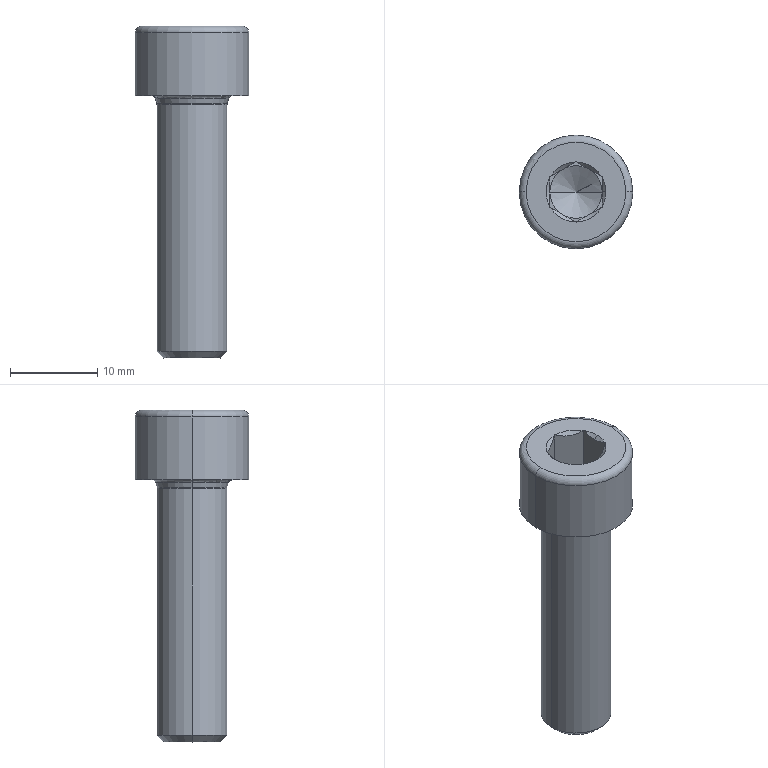Part | NX | features 2_12 2 | 1 solid | 38 faces | box 13 x 13 x 38 mm | volume 2398 mm3 | plane 15 | cone 13 | torus 6 | cylinder 4 | commonest cylinder face diameters 8 x2 13 x2
STEP:
#1=CARTESIAN_POINT('',(-141.767,-145.,-837.129));
#2=VERTEX_POINT('',#1);
#3=CARTESIAN_POINT('',(-148.233,-145.,-837.129));
#4=VERTEX_POINT('',#3);
#5=CARTESIAN_POINT('',(-145.,-145.,-837.129));
#6=DIRECTION('',(0.,0.,-1.));
#7=DIRECTION('',(1.,0.,0.));
#8=AXIS2_PLACEMENT_3D('',#5,#6,#7);
#9=CIRCLE('',#8,3.233);
#10=EDGE_CURVE('',#2,#4,#9,.T.);
#11=ORIENTED_EDGE('',*,*,#10,.F.);
#12=CARTESIAN_POINT('',(-141.,-145.,-836.362));
#13=VERTEX_POINT('',#12);
#14=CARTESIAN_POINT('',(-141.,-145.,-836.362));
#15=DIRECTION('',(-0.7071,0.,-0.7071));
#16=VECTOR('',#15,1000.);
#17=LINE('',#14,#16);
#18=EDGE_CURVE('',#13,#2,#17,.T.);
#19=ORIENTED_EDGE('',*,*,#18,.F.);
#20=CARTESIAN_POINT('',(-149.,-145.,-836.362));
#21=VERTEX_POINT('',#20);
#22=CARTESIAN_POINT('',(-145.,-145.,-836.362));
#23=DIRECTION('',(0.,0.,-1.));
#24=DIRECTION('',(1.,0.,0.));
#25=AXIS2_PLACEMENT_3D('',#22,#23,#24);
#26=CIRCLE('',#25,4.);
#27=EDGE_CURVE('',#13,#21,#26,.T.);
#28=ORIENTED_EDGE('',*,*,#27,.T.);
#29=CARTESIAN_POINT('',(-149.,-145.,-836.362));
#30=DIRECTION('',(0.7071,0.,-0.7071));
#31=VECTOR('',#30,1000.);
#32=LINE('',#29,#31);
#33=EDGE_CURVE('',#4,#21,#32,.F.);
#34=ORIENTED_EDGE('',*,*,#33,.F.);
#35=EDGE_LOOP('',(#11,#19,#28,#34));
#36=FACE_BOUND('',#35,.T.);
#37=CARTESIAN_POINT('',(-145.,-145.,-837.165));
#38=DIRECTION('',(0.,0.,1.));
#39=DIRECTION('',(1.,0.,0.));
#40=AXIS2_PLACEMENT_3D('',#37,#38,#39);
#41=CONICAL_SURFACE('',#40,3.197,0.7854);
#42=ADVANCED_FACE('',(#36),#41,.T.);
#43=ORIENTED_EDGE('',*,*,#10,.T.);
#44=CARTESIAN_POINT('',(-145.,-145.,-837.129));
#45=DIRECTION('',(0.,0.,-1.));
#46=DIRECTION('',(-1.,0.,0.));
#47=AXIS2_PLACEMENT_3D('',#44,#45,#46);
#48=CIRCLE('',#47,3.233);
#49=EDGE_CURVE('',#4,#2,#48,.T.);
#50=ORIENTED_EDGE('',*,*,#49,.T.);
#51=EDGE_LOOP('',(#43,#50));
#52=FACE_BOUND('',#51,.T.);
#53=CARTESIAN_POINT('',(-145.,-146.617,-837.129));
#54=DIRECTION('',(0.,0.,-1.));
#55=DIRECTION('',(-1.,0.,0.));
#56=AXIS2_PLACEMENT_3D('',#53,#54,#55);
#57=PLANE('',#56);
#58=ADVANCED_FACE('',(#52),#57,.T.);
#59=ORIENTED_EDGE('',*,*,#33,.T.);
#60=CARTESIAN_POINT('',(-145.,-145.,-836.362));
#61=DIRECTION('',(0.,0.,-1.));
#62=DIRECTION('',(-1.,0.,0.));
#63=AXIS2_PLACEMENT_3D('',#60,#61,#62);
#64=CIRCLE('',#63,4.);
#65=EDGE_CURVE('',#21,#13,#64,.T.);
#66=ORIENTED_EDGE('',*,*,#65,.T.);
#67=ORIENTED_EDGE('',*,*,#18,.T.);
#68=ORIENTED_EDGE('',*,*,#49,.F.);
#69=EDGE_LOOP('',(#59,#66,#67,#68));
#70=FACE_BOUND('',#69,.T.);
#71=CARTESIAN_POINT('',(-145.,-145.,-837.165));
#72=DIRECTION('',(0.,0.,1.));
#73=DIRECTION('',(1.,0.,0.));
#74=AXIS2_PLACEMENT_3D('',#71,#72,#73);
#75=CONICAL_SURFACE('',#74,3.197,0.7854);
#76=ADVANCED_FACE('',(#70),#75,.T.);
#77=CARTESIAN_POINT('',(-144.94,-141.571,-799.129));
#78=VERTEX_POINT('',#77);
#79=CARTESIAN_POINT('',(-142.06,-143.233,-799.129));
#80=VERTEX_POINT('',#79);
#81=CARTESIAN_POINT('',(-144.94,-141.571,-799.129));
#82=CARTESIAN_POINT('',(-144.491,-141.83,-799.381));
#83=CARTESIAN_POINT('',(-143.5,-142.402,-799.738));
#84=CARTESIAN_POINT('',(-142.509,-142.974,-799.381));
#85=CARTESIAN_POINT('',(-142.06,-143.233,-799.129));
#86=B_SPLINE_CURVE_WITH_KNOTS('',3,(#81,#82,#83,#84,#85),.UNSPECIFIED.,.F.,.F.,(4,1,4),(0.,0.5,1.),.UNSPECIFIED.);
#87=EDGE_CURVE('',#78,#80,#86,.T.);
#88=ORIENTED_EDGE('',*,*,#87,.T.);
#89=CARTESIAN_POINT('',(-145.,-145.,-799.129));
#90=DIRECTION('',(0.,0.,-1.));
#91=DIRECTION('',(0.01749,0.9998,0.));
#92=AXIS2_PLACEMENT_3D('',#89,#90,#91);
#93=CIRCLE('',#92,3.43);
#94=EDGE_CURVE('',#78,#80,#93,.T.);
#95=ORIENTED_EDGE('',*,*,#94,.F.);
#96=EDGE_LOOP('',(#88,#95));
#97=FACE_BOUND('',#96,.T.);
#98=CARTESIAN_POINT('',(-145.,-145.,-799.598));
#99=DIRECTION('',(0.,0.,1.));
#100=DIRECTION('',(1.,0.,0.));
#101=AXIS2_PLACEMENT_3D('',#98,#99,#100);
#102=CONICAL_SURFACE('',#101,2.962,0.7854);
#103=ADVANCED_FACE('',(#97),#102,.F.);
#104=CARTESIAN_POINT('',(-147.94,-143.233,-799.129));
#105=VERTEX_POINT('',#104);
#106=CARTESIAN_POINT('',(-145.06,-141.571,-799.129));
#107=VERTEX_POINT('',#106);
#108=CARTESIAN_POINT('',(-147.94,-143.233,-799.129));
#109=CARTESIAN_POINT('',(-147.491,-142.974,-799.381));
#110=CARTESIAN_POINT('',(-146.5,-142.402,-799.738));
#111=CARTESIAN_POINT('',(-145.509,-141.83,-799.381));
#112=CARTESIAN_POINT('',(-145.06,-141.571,-799.129));
#113=B_SPLINE_CURVE_WITH_KNOTS('',3,(#108,#109,#110,#111,#112),.UNSPECIFIED.,.F.,.F.,(4,1,4),(0.,0.5,1.),.UNSPECIFIED.);
#114=EDGE_CURVE('',#105,#107,#113,.T.);
#115=ORIENTED_EDGE('',*,*,#114,.T.);
#116=CARTESIAN_POINT('',(-145.,-145.,-799.129));
#117=DIRECTION('',(0.,0.,-1.));
#118=DIRECTION('',(-0.8572,0.5151,0.));
#119=AXIS2_PLACEMENT_3D('',#116,#117,#118);
#120=CIRCLE('',#119,3.43);
#121=EDGE_CURVE('',#105,#107,#120,.T.);
#122=ORIENTED_EDGE('',*,*,#121,.F.);
#123=EDGE_LOOP('',(#115,#122));
#124=FACE_BOUND('',#123,.T.);
#125=CARTESIAN_POINT('',(-145.,-145.,-799.598));
#126=DIRECTION('',(0.,0.,1.));
#127=DIRECTION('',(1.,0.,0.));
#128=AXIS2_PLACEMENT_3D('',#125,#126,#127);
#129=CONICAL_SURFACE('',#128,2.962,0.7854);
#130=ADVANCED_FACE('',(#124),#129,.F.);
#131=CARTESIAN_POINT('',(-145.,-141.536,-803.829));
#132=VERTEX_POINT('',#131);
#133=CARTESIAN_POINT('',(-146.5,-142.402,-803.829));
#134=VERTEX_POINT('',#133);
#135=CARTESIAN_POINT('',(-145.,-141.536,-803.829));
#136=DIRECTION('',(-0.866,-0.5,0.));
#137=VECTOR('',#136,1000.);
#138=LINE('',#135,#137);
#139=EDGE_CURVE('',#132,#134,#138,.T.);
#140=ORIENTED_EDGE('',*,*,#139,.T.);
#141=CARTESIAN_POINT('',(-143.5,-142.402,-803.829));
#142=VERTEX_POINT('',#141);
#143=CARTESIAN_POINT('',(-145.,-145.,-803.829));
#144=DIRECTION('',(0.,0.,-1.));
#145=DIRECTION('',(-0.5,0.866,0.));
#146=AXIS2_PLACEMENT_3D('',#143,#144,#145);
#147=CIRCLE('',#146,3.);
#148=EDGE_CURVE('',#134,#142,#147,.T.);
#149=ORIENTED_EDGE('',*,*,#148,.T.);
#150=CARTESIAN_POINT('',(-143.5,-142.402,-803.829));
#151=DIRECTION('',(-0.866,0.5,0.));
#152=VECTOR('',#151,1000.);
#153=LINE('',#150,#152);
#154=EDGE_CURVE('',#142,#132,#153,.T.);
#155=ORIENTED_EDGE('',*,*,#154,.T.);
#156=EDGE_LOOP('',(#140,#149,#155));
#157=FACE_BOUND('',#156,.T.);
#158=CARTESIAN_POINT('',(-145.,-145.,-803.829));
#159=DIRECTION('',(0.,0.,-1.));
#160=DIRECTION('',(-1.,0.,0.));
#161=AXIS2_PLACEMENT_3D('',#158,#159,#160);
#162=PLANE('',#161);
#163=ADVANCED_FACE('',(#157),#162,.F.);
#164=CARTESIAN_POINT('',(-145.,-148.464,-803.829));
#165=VERTEX_POINT('',#164);
#166=CARTESIAN_POINT('',(-143.5,-147.598,-803.829));
#167=VERTEX_POINT('',#166);
#168=CARTESIAN_POINT('',(-145.,-148.464,-803.829));
#169=DIRECTION('',(0.866,0.5,0.));
#170=VECTOR('',#169,1000.);
#171=LINE('',#168,#170);
#172=EDGE_CURVE('',#165,#167,#171,.T.);
#173=ORIENTED_EDGE('',*,*,#172,.T.);
#174=CARTESIAN_POINT('',(-146.5,-147.598,-803.829));
#175=VERTEX_POINT('',#174);
#176=CARTESIAN_POINT('',(-145.,-145.,-803.829));
#177=DIRECTION('',(0.,0.,-1.));
#178=DIRECTION('',(0.5,-0.866,0.));
#179=AXIS2_PLACEMENT_3D('',#176,#177,#178);
#180=CIRCLE('',#179,3.);
#181=EDGE_CURVE('',#167,#175,#180,.T.);
#182=ORIENTED_EDGE('',*,*,#181,.T.);
#183=CARTESIAN_POINT('',(-146.5,-147.598,-803.829));
#184=DIRECTION('',(0.866,-0.5,0.));
#185=VECTOR('',#184,1000.);
#186=LINE('',#183,#185);
#187=EDGE_CURVE('',#175,#165,#186,.T.);
#188=ORIENTED_EDGE('',*,*,#187,.T.);
#189=EDGE_LOOP('',(#173,#182,#188));
#190=FACE_BOUND('',#189,.T.);
#191=CARTESIAN_POINT('',(-145.,-145.,-803.829));
#192=DIRECTION('',(0.,0.,-1.));
#193=DIRECTION('',(-1.,0.,0.));
#194=AXIS2_PLACEMENT_3D('',#191,#192,#193);
#195=PLANE('',#194);
#196=ADVANCED_FACE('',(#190),#195,.F.);
#197=CARTESIAN_POINT('',(-148.,-146.732,-803.829));
#198=VERTEX_POINT('',#197);
#199=CARTESIAN_POINT('',(-148.,-146.732,-803.829));
#200=DIRECTION('',(0.866,-0.5,0.));
#201=VECTOR('',#200,1000.);
#202=LINE('',#199,#201);
#203=EDGE_CURVE('',#198,#175,#202,.T.);
#204=ORIENTED_EDGE('',*,*,#203,.T.);
#205=CARTESIAN_POINT('',(-148.,-145.,-803.829));
#206=VERTEX_POINT('',#205);
#207=CARTESIAN_POINT('',(-145.,-145.,-803.829));
#208=DIRECTION('',(0.,0.,-1.));
#209=DIRECTION('',(-0.5,-0.866,0.));
#210=AXIS2_PLACEMENT_3D('',#207,#208,#209);
#211=CIRCLE('',#210,3.);
#212=EDGE_CURVE('',#175,#206,#211,.T.);
#213=ORIENTED_EDGE('',*,*,#212,.T.);
#214=CARTESIAN_POINT('',(-148.,-145.,-803.829));
#215=DIRECTION('',(0.,-1.,0.));
#216=VECTOR('',#215,1000.);
#217=LINE('',#214,#216);
#218=EDGE_CURVE('',#206,#198,#217,.T.);
#219=ORIENTED_EDGE('',*,*,#218,.T.);
#220=EDGE_LOOP('',(#204,#213,#219));
#221=FACE_BOUND('',#220,.T.);
#222=CARTESIAN_POINT('',(-145.,-145.,-803.829));
#223=DIRECTION('',(0.,0.,-1.));
#224=DIRECTION('',(-1.,0.,0.));
#225=AXIS2_PLACEMENT_3D('',#222,#223,#224);
#226=PLANE('',#225);
#227=ADVANCED_FACE('',(#221),#226,.F.);
#228=CARTESIAN_POINT('',(-145.06,-148.429,-799.129));
#229=VERTEX_POINT('',#228);
#230=CARTESIAN_POINT('',(-147.94,-146.767,-799.129));
#231=VERTEX_POINT('',#230);
#232=CARTESIAN_POINT('',(-145.,-145.,-799.129));
#233=DIRECTION('',(0.,0.,-1.));
#234=DIRECTION('',(-0.01749,-0.9998,0.));
#235=AXIS2_PLACEMENT_3D('',#232,#233,#234);
#236=CIRCLE('',#235,3.43);
#237=EDGE_CURVE('',#229,#231,#236,.T.);
#238=ORIENTED_EDGE('',*,*,#237,.F.);
#239=CARTESIAN_POINT('',(-145.06,-148.429,-799.129));
#240=CARTESIAN_POINT('',(-145.509,-148.17,-799.381));
#241=CARTESIAN_POINT('',(-146.5,-147.598,-799.738));
#242=CARTESIAN_POINT('',(-147.491,-147.026,-799.381));
#243=CARTESIAN_POINT('',(-147.94,-146.767,-799.129));
#244=B_SPLINE_CURVE_WITH_KNOTS('',3,(#239,#240,#241,#242,#243),.UNSPECIFIED.,.F.,.F.,(4,1,4),(0.,0.5,1.),.UNSPECIFIED.);
#245=EDGE_CURVE('',#229,#231,#244,.T.);
#246=ORIENTED_EDGE('',*,*,#245,.T.);
#247=EDGE_LOOP('',(#238,#246));
#248=FACE_BOUND('',#247,.T.);
#249=CARTESIAN_POINT('',(-145.,-145.,-799.598));
#250=DIRECTION('',(0.,0.,1.));
#251=DIRECTION('',(1.,0.,0.));
#252=AXIS2_PLACEMENT_3D('',#249,#250,#251);
#253=CONICAL_SURFACE('',#252,2.962,0.7854);
#254=ADVANCED_FACE('',(#248),#253,.F.);
#255=ORIENTED_EDGE('',*,*,#187,.F.);
#256=ORIENTED_EDGE('',*,*,#203,.F.);
#257=CARTESIAN_POINT('',(-148.,-146.732,-799.129));
#258=VERTEX_POINT('',#257);
#259=CARTESIAN_POINT('',(-148.,-146.732,-799.129));
#260=DIRECTION('',(0.,0.,-1.));
#261=VECTOR('',#260,1000.);
#262=LINE('',#259,#261);
#263=EDGE_CURVE('',#258,#198,#262,.T.);
#264=ORIENTED_EDGE('',*,*,#263,.F.);
#265=CARTESIAN_POINT('',(-147.94,-146.767,-799.129));
#266=DIRECTION('',(-0.866,0.5,0.));
#267=VECTOR('',#266,1000.);
#268=LINE('',#265,#267);
#269=EDGE_CURVE('',#231,#258,#268,.T.);
#270=ORIENTED_EDGE('',*,*,#269,.F.);
#271=ORIENTED_EDGE('',*,*,#245,.F.);
#272=CARTESIAN_POINT('',(-145.,-148.464,-799.129));
#273=VERTEX_POINT('',#272);
#274=CARTESIAN_POINT('',(-145.,-148.464,-799.129));
#275=DIRECTION('',(-0.866,0.5,0.));
#276=VECTOR('',#275,1000.);
#277=LINE('',#274,#276);
#278=EDGE_CURVE('',#273,#229,#277,.T.);
#279=ORIENTED_EDGE('',*,*,#278,.F.);
#280=CARTESIAN_POINT('',(-145.,-148.464,-799.129));
#281=DIRECTION('',(0.,0.,-1.));
#282=VECTOR('',#281,1000.);
#283=LINE('',#280,#282);
#284=EDGE_CURVE('',#273,#165,#283,.T.);
#285=ORIENTED_EDGE('',*,*,#284,.T.);
#286=EDGE_LOOP('',(#255,#256,#264,#270,#271,#279,#285));
#287=FACE_BOUND('',#286,.T.);
#288=CARTESIAN_POINT('',(-145.,-148.464,-803.829));
#289=DIRECTION('',(-0.5,-0.866,0.));
#290=DIRECTION('',(0.866,-0.5,0.));
#291=AXIS2_PLACEMENT_3D('',#288,#289,#290);
#292=PLANE('',#291);
#293=ADVANCED_FACE('',(#287),#292,.F.);
#294=CARTESIAN_POINT('',(-142.06,-146.767,-799.129));
#295=VERTEX_POINT('',#294);
#296=CARTESIAN_POINT('',(-144.94,-148.429,-799.129));
#297=VERTEX_POINT('',#296);
#298=CARTESIAN_POINT('',(-145.,-145.,-799.129));
#299=DIRECTION('',(0.,0.,-1.));
#300=DIRECTION('',(0.8572,-0.5151,0.));
#301=AXIS2_PLACEMENT_3D('',#298,#299,#300);
#302=CIRCLE('',#301,3.43);
#303=EDGE_CURVE('',#295,#297,#302,.T.);
#304=ORIENTED_EDGE('',*,*,#303,.F.);
#305=CARTESIAN_POINT('',(-142.06,-146.767,-799.129));
#306=CARTESIAN_POINT('',(-142.509,-147.026,-799.381));
#307=CARTESIAN_POINT('',(-143.5,-147.598,-799.738));
#308=CARTESIAN_POINT('',(-144.491,-148.17,-799.381));
#309=CARTESIAN_POINT('',(-144.94,-148.429,-799.129));
#310=B_SPLINE_CURVE_WITH_KNOTS('',3,(#305,#306,#307,#308,#309),.UNSPECIFIED.,.F.,.F.,(4,1,4),(0.,0.5,1.),.UNSPECIFIED.);
#311=EDGE_CURVE('',#295,#297,#310,.T.);
#312=ORIENTED_EDGE('',*,*,#311,.T.);
#313=EDGE_LOOP('',(#304,#312));
#314=FACE_BOUND('',#313,.T.);
#315=CARTESIAN_POINT('',(-145.,-145.,-799.598));
#316=DIRECTION('',(0.,0.,1.));
#317=DIRECTION('',(1.,0.,0.));
#318=AXIS2_PLACEMENT_3D('',#315,#316,#317);
#319=CONICAL_SURFACE('',#318,2.962,0.7854);
#320=ADVANCED_FACE('',(#314),#319,.F.);
#321=CARTESIAN_POINT('',(-142.,-143.268,-803.829));
#322=VERTEX_POINT('',#321);
#323=CARTESIAN_POINT('',(-142.,-143.268,-803.829));
#324=DIRECTION('',(-0.866,0.5,0.));
#325=VECTOR('',#324,1000.);
#326=LINE('',#323,#325);
#327=EDGE_CURVE('',#322,#142,#326,.T.);
#328=ORIENTED_EDGE('',*,*,#327,.T.);
#329=CARTESIAN_POINT('',(-142.,-145.,-803.829));
#330=VERTEX_POINT('',#329);
#331=CARTESIAN_POINT('',(-145.,-145.,-803.829));
#332=DIRECTION('',(0.,0.,-1.));
#333=DIRECTION('',(0.5,0.866,0.));
#334=AXIS2_PLACEMENT_3D('',#331,#332,#333);
#335=CIRCLE('',#334,3.);
#336=EDGE_CURVE('',#142,#330,#335,.T.);
#337=ORIENTED_EDGE('',*,*,#336,.T.);
#338=CARTESIAN_POINT('',(-142.,-145.,-803.829));
#339=DIRECTION('',(0.,1.,0.));
#340=VECTOR('',#339,1000.);
#341=LINE('',#338,#340);
#342=EDGE_CURVE('',#330,#322,#341,.T.);
#343=ORIENTED_EDGE('',*,*,#342,.T.);
#344=EDGE_LOOP('',(#328,#337,#343));
#345=FACE_BOUND('',#344,.T.);
#346=CARTESIAN_POINT('',(-145.,-145.,-803.829));
#347=DIRECTION('',(0.,0.,-1.));
#348=DIRECTION('',(-1.,0.,0.));
#349=AXIS2_PLACEMENT_3D('',#346,#347,#348);
#350=PLANE('',#349);
#351=ADVANCED_FACE('',(#345),#350,.F.);
#352=CARTESIAN_POINT('',(-142.,-145.,-799.559));
#353=VERTEX_POINT('',#352);
#354=CARTESIAN_POINT('',(-142.,-146.663,-799.129));
#355=VERTEX_POINT('',#354);
#356=CARTESIAN_POINT('',(-142.,-145.,-799.559));
#357=CARTESIAN_POINT('',(-142.,-145.578,-799.561));
#358=CARTESIAN_POINT('',(-142.,-146.144,-799.381));
#359=CARTESIAN_POINT('',(-142.,-146.663,-799.129));
#360=B_SPLINE_CURVE_WITH_KNOTS('',3,(#356,#357,#358,#359),.UNSPECIFIED.,.F.,.F.,(4,4),(0.,1.),.UNSPECIFIED.);
#361=EDGE_CURVE('',#353,#355,#360,.T.);
#362=ORIENTED_EDGE('',*,*,#361,.T.);
#363=CARTESIAN_POINT('',(-141.57,-145.,-799.129));
#364=VERTEX_POINT('',#363);
#365=CARTESIAN_POINT('',(-145.,-145.,-799.129));
#366=DIRECTION('',(0.,0.,-1.));
#367=DIRECTION('',(1.,0.,0.));
#368=AXIS2_PLACEMENT_3D('',#365,#366,#367);
#369=CIRCLE('',#368,3.43);
#370=EDGE_CURVE('',#364,#355,#369,.T.);
#371=ORIENTED_EDGE('',*,*,#370,.F.);
#372=CARTESIAN_POINT('',(-141.57,-145.,-799.129));
#373=DIRECTION('',(-0.7071,0.,-0.7071));
#374=VECTOR('',#373,1000.);
#375=LINE('',#372,#374);
#376=EDGE_CURVE('',#364,#353,#375,.T.);
#377=ORIENTED_EDGE('',*,*,#376,.T.);
#378=EDGE_LOOP('',(#362,#371,#377));
#379=FACE_BOUND('',#378,.T.);
#380=CARTESIAN_POINT('',(-145.,-145.,-799.595));
#381=DIRECTION('',(0.,0.,1.));
#382=DIRECTION('',(1.,0.,0.));
#383=AXIS2_PLACEMENT_3D('',#380,#381,#382);
#384=CONICAL_SURFACE('',#383,2.964,0.7854);
#385=ADVANCED_FACE('',(#379),#384,.F.);
#386=ORIENTED_EDGE('',*,*,#376,.F.);
#387=CARTESIAN_POINT('',(-142.,-143.337,-799.129));
#388=VERTEX_POINT('',#387);
#389=CARTESIAN_POINT('',(-145.,-145.,-799.129));
#390=DIRECTION('',(0.,0.,-1.));
#391=DIRECTION('',(0.8746,0.4848,0.));
#392=AXIS2_PLACEMENT_3D('',#389,#390,#391);
#393=CIRCLE('',#392,3.43);
#394=EDGE_CURVE('',#388,#364,#393,.T.);
#395=ORIENTED_EDGE('',*,*,#394,.F.);
#396=CARTESIAN_POINT('',(-142.,-143.337,-799.129));
#397=CARTESIAN_POINT('',(-142.,-143.856,-799.381));
#398=CARTESIAN_POINT('',(-142.,-144.422,-799.56));
#399=CARTESIAN_POINT('',(-142.,-145.,-799.559));
#400=B_SPLINE_CURVE_WITH_KNOTS('',3,(#396,#397,#398,#399),.UNSPECIFIED.,.F.,.F.,(4,4),(0.,1.),.UNSPECIFIED.);
#401=EDGE_CURVE('',#388,#353,#400,.T.);
#402=ORIENTED_EDGE('',*,*,#401,.T.);
#403=EDGE_LOOP('',(#386,#395,#402));
#404=FACE_BOUND('',#403,.T.);
#405=CARTESIAN_POINT('',(-145.,-145.,-799.595));
#406=DIRECTION('',(0.,0.,1.));
#407=DIRECTION('',(1.,0.,0.));
#408=AXIS2_PLACEMENT_3D('',#405,#406,#407);
#409=CONICAL_SURFACE('',#408,2.964,0.7854);
#410=ADVANCED_FACE('',(#404),#409,.F.);
#411=ORIENTED_EDGE('',*,*,#342,.F.);
#412=CARTESIAN_POINT('',(-142.,-146.732,-803.829));
#413=VERTEX_POINT('',#412);
#414=CARTESIAN_POINT('',(-142.,-145.,-803.829));
#415=DIRECTION('',(0.,-1.,0.));
#416=VECTOR('',#415,1000.);
#417=LINE('',#414,#416);
#418=EDGE_CURVE('',#330,#413,#417,.T.);
#419=ORIENTED_EDGE('',*,*,#418,.T.);
#420=CARTESIAN_POINT('',(-142.,-146.732,-799.129));
#421=VERTEX_POINT('',#420);
#422=CARTESIAN_POINT('',(-142.,-146.732,-799.129));
#423=DIRECTION('',(0.,0.,-1.));
#424=VECTOR('',#423,1000.);
#425=LINE('',#422,#424);
#426=EDGE_CURVE('',#421,#413,#425,.T.);
#427=ORIENTED_EDGE('',*,*,#426,.F.);
#428=CARTESIAN_POINT('',(-142.,-146.732,-799.129));
#429=DIRECTION('',(0.,1.,0.));
#430=VECTOR('',#429,1000.);
#431=LINE('',#428,#430);
#432=EDGE_CURVE('',#421,#355,#431,.T.);
#433=ORIENTED_EDGE('',*,*,#432,.T.);
#434=ORIENTED_EDGE('',*,*,#361,.F.);
#435=ORIENTED_EDGE('',*,*,#401,.F.);
#436=CARTESIAN_POINT('',(-142.,-143.268,-799.129));
#437=VERTEX_POINT('',#436);
#438=CARTESIAN_POINT('',(-142.,-143.337,-799.129));
#439=DIRECTION('',(0.,1.,0.));
#440=VECTOR('',#439,1000.);
#441=LINE('',#438,#440);
#442=EDGE_CURVE('',#388,#437,#441,.T.);
#443=ORIENTED_EDGE('',*,*,#442,.T.);
#444=CARTESIAN_POINT('',(-142.,-143.268,-803.829));
#445=DIRECTION('',(0.,0.,1.));
#446=VECTOR('',#445,1000.);
#447=LINE('',#444,#446);
#448=EDGE_CURVE('',#322,#437,#447,.T.);
#449=ORIENTED_EDGE('',*,*,#448,.F.);
#450=EDGE_LOOP('',(#411,#419,#427,#433,#434,#435,#443,#449));
#451=FACE_BOUND('',#450,.T.);
#452=CARTESIAN_POINT('',(-142.,-143.268,-803.829));
#453=DIRECTION('',(1.,0.,0.));
#454=DIRECTION('',(0.,0.,-1.));
#455=AXIS2_PLACEMENT_3D('',#452,#453,#454);
#456=PLANE('',#455);
#457=ADVANCED_FACE('',(#451),#456,.F.);
#458=CARTESIAN_POINT('',(-143.5,-147.598,-803.829));
#459=DIRECTION('',(0.866,0.5,0.));
#460=VECTOR('',#459,1000.);
#461=LINE('',#458,#460);
#462=EDGE_CURVE('',#167,#413,#461,.T.);
#463=ORIENTED_EDGE('',*,*,#462,.F.);
#464=ORIENTED_EDGE('',*,*,#172,.F.);
#465=ORIENTED_EDGE('',*,*,#284,.F.);
#466=CARTESIAN_POINT('',(-144.94,-148.429,-799.129));
#467=DIRECTION('',(-0.866,-0.5,0.));
#468=VECTOR('',#467,1000.);
#469=LINE('',#466,#468);
#470=EDGE_CURVE('',#297,#273,#469,.T.);
#471=ORIENTED_EDGE('',*,*,#470,.F.);
#472=ORIENTED_EDGE('',*,*,#311,.F.);
#473=CARTESIAN_POINT('',(-142.,-146.732,-799.129));
#474=DIRECTION('',(-0.866,-0.5,0.));
#475=VECTOR('',#474,1000.);
#476=LINE('',#473,#475);
#477=EDGE_CURVE('',#421,#295,#476,.T.);
#478=ORIENTED_EDGE('',*,*,#477,.F.);
#479=ORIENTED_EDGE('',*,*,#426,.T.);
#480=EDGE_LOOP('',(#463,#464,#465,#471,#472,#478,#479));
#481=FACE_BOUND('',#480,.T.);
#482=CARTESIAN_POINT('',(-142.,-146.732,-803.829));
#483=DIRECTION('',(0.5,-0.866,0.));
#484=DIRECTION('',(0.866,0.5,0.));
#485=AXIS2_PLACEMENT_3D('',#482,#483,#484);
#486=PLANE('',#485);
#487=ADVANCED_FACE('',(#481),#486,.F.);
#488=ORIENTED_EDGE('',*,*,#418,.F.);
#489=CARTESIAN_POINT('',(-145.,-145.,-803.829));
#490=DIRECTION('',(0.,0.,-1.));
#491=DIRECTION('',(1.,0.,0.));
#492=AXIS2_PLACEMENT_3D('',#489,#490,#491);
#493=CIRCLE('',#492,3.);
#494=EDGE_CURVE('',#330,#167,#493,.T.);
#495=ORIENTED_EDGE('',*,*,#494,.T.);
#496=ORIENTED_EDGE('',*,*,#462,.T.);
#497=EDGE_LOOP('',(#488,#495,#496));
#498=FACE_BOUND('',#497,.T.);
#499=CARTESIAN_POINT('',(-145.,-145.,-803.829));
#500=DIRECTION('',(0.,0.,-1.));
#501=DIRECTION('',(-1.,0.,0.));
#502=AXIS2_PLACEMENT_3D('',#499,#500,#501);
#503=PLANE('',#502);
#504=ADVANCED_FACE('',(#498),#503,.F.);
#505=CARTESIAN_POINT('',(-145.,-145.,-805.561));
#506=VERTEX_POINT('',#505);
#507=CARTESIAN_POINT('',(-148.,-145.,-803.829));
#508=DIRECTION('',(0.866,0.,-0.5));
#509=VECTOR('',#508,1000.);
#510=LINE('',#507,#509);
#511=EDGE_CURVE('',#206,#506,#510,.T.);
#512=ORIENTED_EDGE('',*,*,#511,.F.);
#513=ORIENTED_EDGE('',*,*,#212,.F.);
#514=ORIENTED_EDGE('',*,*,#181,.F.);
#515=ORIENTED_EDGE('',*,*,#494,.F.);
#516=CARTESIAN_POINT('',(-142.,-145.,-803.829));
#517=DIRECTION('',(-0.866,0.,-0.5));
#518=VECTOR('',#517,1000.);
#519=LINE('',#516,#518);
#520=EDGE_CURVE('',#506,#330,#519,.F.);
#521=ORIENTED_EDGE('',*,*,#520,.F.);
#522=EDGE_LOOP('',(#512,#513,#514,#515,#521));
#523=FACE_BOUND('',#522,.T.);
#524=CARTESIAN_POINT('',(-145.,-145.,-805.561));
#525=DIRECTION('',(0.,0.,1.));
#526=DIRECTION('',(1.,0.,0.));
#527=AXIS2_PLACEMENT_3D('',#524,#525,#526);
#528=CONICAL_SURFACE('',#527,0.,1.047);
#529=ADVANCED_FACE('',(#523),#528,.F.);
#530=ORIENTED_EDGE('',*,*,#520,.T.);
#531=ORIENTED_EDGE('',*,*,#336,.F.);
#532=ORIENTED_EDGE('',*,*,#148,.F.);
#533=CARTESIAN_POINT('',(-145.,-145.,-803.829));
#534=DIRECTION('',(0.,0.,-1.));
#535=DIRECTION('',(-1.,0.,0.));
#536=AXIS2_PLACEMENT_3D('',#533,#534,#535);
#537=CIRCLE('',#536,3.);
#538=EDGE_CURVE('',#206,#134,#537,.T.);
#539=ORIENTED_EDGE('',*,*,#538,.F.);
#540=ORIENTED_EDGE('',*,*,#511,.T.);
#541=EDGE_LOOP('',(#530,#531,#532,#539,#540));
#542=FACE_BOUND('',#541,.T.);
#543=CARTESIAN_POINT('',(-145.,-145.,-805.561));
#544=DIRECTION('',(0.,0.,1.));
#545=DIRECTION('',(1.,0.,0.));
#546=AXIS2_PLACEMENT_3D('',#543,#544,#545);
#547=CONICAL_SURFACE('',#546,0.,1.047);
#548=ADVANCED_FACE('',(#542),#547,.F.);
#549=CARTESIAN_POINT('',(-148.,-143.268,-803.829));
#550=VERTEX_POINT('',#549);
#551=CARTESIAN_POINT('',(-148.,-143.268,-803.829));
#552=DIRECTION('',(0.,-1.,0.));
#553=VECTOR('',#552,1000.);
#554=LINE('',#551,#553);
#555=EDGE_CURVE('',#550,#206,#554,.T.);
#556=ORIENTED_EDGE('',*,*,#555,.T.);
#557=ORIENTED_EDGE('',*,*,#538,.T.);
#558=CARTESIAN_POINT('',(-146.5,-142.402,-803.829));
#559=DIRECTION('',(-0.866,-0.5,0.));
#560=VECTOR('',#559,1000.);
#561=LINE('',#558,#560);
#562=EDGE_CURVE('',#134,#550,#561,.T.);
#563=ORIENTED_EDGE('',*,*,#562,.T.);
#564=EDGE_LOOP('',(#556,#557,#563));
#565=FACE_BOUND('',#564,.T.);
#566=CARTESIAN_POINT('',(-145.,-145.,-803.829));
#567=DIRECTION('',(0.,0.,-1.));
#568=DIRECTION('',(-1.,0.,0.));
#569=AXIS2_PLACEMENT_3D('',#566,#567,#568);
#570=PLANE('',#569);
#571=ADVANCED_FACE('',(#565),#570,.F.);
#572=CARTESIAN_POINT('',(-148.,-146.663,-799.129));
#573=VERTEX_POINT('',#572);
#574=CARTESIAN_POINT('',(-148.43,-145.,-799.129));
#575=VERTEX_POINT('',#574);
#576=CARTESIAN_POINT('',(-145.,-145.,-799.129));
#577=DIRECTION('',(0.,0.,-1.));
#578=DIRECTION('',(-0.8746,-0.4848,0.));
#579=AXIS2_PLACEMENT_3D('',#576,#577,#578);
#580=CIRCLE('',#579,3.43);
#581=EDGE_CURVE('',#573,#575,#580,.T.);
#582=ORIENTED_EDGE('',*,*,#581,.F.);
#583=CARTESIAN_POINT('',(-148.,-145.,-799.559));
#584=VERTEX_POINT('',#583);
#585=CARTESIAN_POINT('',(-148.,-146.663,-799.129));
#586=CARTESIAN_POINT('',(-148.,-146.144,-799.381));
#587=CARTESIAN_POINT('',(-148.,-145.578,-799.56));
#588=CARTESIAN_POINT('',(-148.,-145.,-799.559));
#589=B_SPLINE_CURVE_WITH_KNOTS('',3,(#585,#586,#587,#588),.UNSPECIFIED.,.F.,.F.,(4,4),(0.,1.),.UNSPECIFIED.);
#590=EDGE_CURVE('',#573,#584,#589,.T.);
#591=ORIENTED_EDGE('',*,*,#590,.T.);
#592=CARTESIAN_POINT('',(-148.,-143.337,-799.129));
#593=VERTEX_POINT('',#592);
#594=CARTESIAN_POINT('',(-148.,-145.,-799.559));
#595=CARTESIAN_POINT('',(-148.,-144.422,-799.561));
#596=CARTESIAN_POINT('',(-148.,-143.856,-799.381));
#597=CARTESIAN_POINT('',(-148.,-143.337,-799.129));
#598=B_SPLINE_CURVE_WITH_KNOTS('',3,(#594,#595,#596,#597),.UNSPECIFIED.,.F.,.F.,(4,4),(0.,1.),.UNSPECIFIED.);
#599=EDGE_CURVE('',#584,#593,#598,.T.);
#600=ORIENTED_EDGE('',*,*,#599,.T.);
#601=CARTESIAN_POINT('',(-145.,-145.,-799.129));
#602=DIRECTION('',(0.,0.,-1.));
#603=DIRECTION('',(-1.,0.,0.));
#604=AXIS2_PLACEMENT_3D('',#601,#602,#603);
#605=CIRCLE('',#604,3.43);
#606=EDGE_CURVE('',#575,#593,#605,.T.);
#607=ORIENTED_EDGE('',*,*,#606,.F.);
#608=EDGE_LOOP('',(#582,#591,#600,#607));
#609=FACE_BOUND('',#608,.T.);
#610=CARTESIAN_POINT('',(-145.,-145.,-799.595));
#611=DIRECTION('',(0.,0.,1.));
#612=DIRECTION('',(1.,0.,0.));
#613=AXIS2_PLACEMENT_3D('',#610,#611,#612);
#614=CONICAL_SURFACE('',#613,2.964,0.7854);
#615=ADVANCED_FACE('',(#609),#614,.F.);
#616=ORIENTED_EDGE('',*,*,#263,.T.);
#617=ORIENTED_EDGE('',*,*,#218,.F.);
#618=ORIENTED_EDGE('',*,*,#555,.F.);
#619=CARTESIAN_POINT('',(-148.,-143.268,-799.129));
#620=VERTEX_POINT('',#619);
#621=CARTESIAN_POINT('',(-148.,-143.268,-799.129));
#622=DIRECTION('',(0.,0.,-1.));
#623=VECTOR('',#622,1000.);
#624=LINE('',#621,#623);
#625=EDGE_CURVE('',#620,#550,#624,.T.);
#626=ORIENTED_EDGE('',*,*,#625,.F.);
#627=CARTESIAN_POINT('',(-148.,-143.268,-799.129));
#628=DIRECTION('',(0.,-1.,0.));
#629=VECTOR('',#628,1000.);
#630=LINE('',#627,#629);
#631=EDGE_CURVE('',#620,#593,#630,.T.);
#632=ORIENTED_EDGE('',*,*,#631,.T.);
#633=ORIENTED_EDGE('',*,*,#599,.F.);
#634=ORIENTED_EDGE('',*,*,#590,.F.);
#635=CARTESIAN_POINT('',(-148.,-146.663,-799.129));
#636=DIRECTION('',(0.,-1.,0.));
#637=VECTOR('',#636,1000.);
#638=LINE('',#635,#637);
#639=EDGE_CURVE('',#573,#258,#638,.T.);
#640=ORIENTED_EDGE('',*,*,#639,.T.);
#641=EDGE_LOOP('',(#616,#617,#618,#626,#632,#633,#634,#640));
#642=FACE_BOUND('',#641,.T.);
#643=CARTESIAN_POINT('',(-148.,-146.732,-803.829));
#644=DIRECTION('',(-1.,0.,0.));
#645=DIRECTION('',(0.,0.,1.));
#646=AXIS2_PLACEMENT_3D('',#643,#644,#645);
#647=PLANE('',#646);
#648=ADVANCED_FACE('',(#642),#647,.F.);
#649=ORIENTED_EDGE('',*,*,#562,.F.);
#650=ORIENTED_EDGE('',*,*,#139,.F.);
#651=CARTESIAN_POINT('',(-145.,-141.536,-799.129));
#652=VERTEX_POINT('',#651);
#653=CARTESIAN_POINT('',(-145.,-141.536,-799.129));
#654=DIRECTION('',(0.,0.,-1.));
#655=VECTOR('',#654,1000.);
#656=LINE('',#653,#655);
#657=EDGE_CURVE('',#652,#132,#656,.T.);
#658=ORIENTED_EDGE('',*,*,#657,.F.);
#659=CARTESIAN_POINT('',(-145.06,-141.571,-799.129));
#660=DIRECTION('',(0.866,0.5,0.));
#661=VECTOR('',#660,1000.);
#662=LINE('',#659,#661);
#663=EDGE_CURVE('',#107,#652,#662,.T.);
#664=ORIENTED_EDGE('',*,*,#663,.F.);
#665=ORIENTED_EDGE('',*,*,#114,.F.);
#666=CARTESIAN_POINT('',(-148.,-143.268,-799.129));
#667=DIRECTION('',(0.866,0.5,0.));
#668=VECTOR('',#667,1000.);
#669=LINE('',#666,#668);
#670=EDGE_CURVE('',#620,#105,#669,.T.);
#671=ORIENTED_EDGE('',*,*,#670,.F.);
#672=ORIENTED_EDGE('',*,*,#625,.T.);
#673=EDGE_LOOP('',(#649,#650,#658,#664,#665,#671,#672));
#674=FACE_BOUND('',#673,.T.);
#675=CARTESIAN_POINT('',(-148.,-143.268,-803.829));
#676=DIRECTION('',(-0.5,0.866,0.));
#677=DIRECTION('',(-0.866,-0.5,0.));
#678=AXIS2_PLACEMENT_3D('',#675,#676,#677);
#679=PLANE('',#678);
#680=ADVANCED_FACE('',(#674),#679,.F.);
#681=ORIENTED_EDGE('',*,*,#154,.F.);
#682=ORIENTED_EDGE('',*,*,#327,.F.);
#683=ORIENTED_EDGE('',*,*,#448,.T.);
#684=CARTESIAN_POINT('',(-142.06,-143.233,-799.129));
#685=DIRECTION('',(0.866,-0.5,0.));
#686=VECTOR('',#685,1000.);
#687=LINE('',#684,#686);
#688=EDGE_CURVE('',#80,#437,#687,.T.);
#689=ORIENTED_EDGE('',*,*,#688,.F.);
#690=ORIENTED_EDGE('',*,*,#87,.F.);
#691=CARTESIAN_POINT('',(-145.,-141.536,-799.129));
#692=DIRECTION('',(0.866,-0.5,0.));
#693=VECTOR('',#692,1000.);
#694=LINE('',#691,#693);
#695=EDGE_CURVE('',#652,#78,#694,.T.);
#696=ORIENTED_EDGE('',*,*,#695,.F.);
#697=ORIENTED_EDGE('',*,*,#657,.T.);
#698=EDGE_LOOP('',(#681,#682,#683,#689,#690,#696,#697));
#699=FACE_BOUND('',#698,.T.);
#700=CARTESIAN_POINT('',(-145.,-141.536,-803.829));
#701=DIRECTION('',(0.5,0.866,0.));
#702=DIRECTION('',(-0.866,0.5,0.));
#703=AXIS2_PLACEMENT_3D('',#700,#701,#702);
#704=PLANE('',#703);
#705=ADVANCED_FACE('',(#699),#704,.F.);
#706=CARTESIAN_POINT('',(-151.5,-145.,-799.929));
#707=VERTEX_POINT('',#706);
#708=CARTESIAN_POINT('',(-138.5,-145.,-799.929));
#709=VERTEX_POINT('',#708);
#710=CARTESIAN_POINT('',(-145.,-145.,-799.929));
#711=DIRECTION('',(0.,0.,1.));
#712=DIRECTION('',(-1.,0.,0.));
#713=AXIS2_PLACEMENT_3D('',#710,#711,#712);
#714=CIRCLE('',#713,6.5);
#715=EDGE_CURVE('',#707,#709,#714,.T.);
#716=ORIENTED_EDGE('',*,*,#715,.F.);
#717=CARTESIAN_POINT('',(-151.5,-145.,-807.129));
#718=VERTEX_POINT('',#717);
#719=CARTESIAN_POINT('',(-151.5,-145.,-807.129));
#720=DIRECTION('',(0.,0.,1.));
#721=VECTOR('',#720,1000.);
#722=LINE('',#719,#721);
#723=EDGE_CURVE('',#718,#707,#722,.T.);
#724=ORIENTED_EDGE('',*,*,#723,.F.);
#725=CARTESIAN_POINT('',(-138.5,-145.,-807.129));
#726=VERTEX_POINT('',#725);
#727=CARTESIAN_POINT('',(-145.,-145.,-807.129));
#728=DIRECTION('',(0.,0.,-1.));
#729=DIRECTION('',(1.,0.,0.));
#730=AXIS2_PLACEMENT_3D('',#727,#728,#729);
#731=CIRCLE('',#730,6.5);
#732=EDGE_CURVE('',#726,#718,#731,.T.);
#733=ORIENTED_EDGE('',*,*,#732,.F.);
#734=CARTESIAN_POINT('',(-138.5,-145.,-807.129));
#735=DIRECTION('',(0.,0.,1.));
#736=VECTOR('',#735,1000.);
#737=LINE('',#734,#736);
#738=EDGE_CURVE('',#709,#726,#737,.F.);
#739=ORIENTED_EDGE('',*,*,#738,.F.);
#740=EDGE_LOOP('',(#716,#724,#733,#739));
#741=FACE_BOUND('',#740,.T.);
#742=CARTESIAN_POINT('',(-145.,-145.,-803.529));
#743=DIRECTION('',(0.,0.,-1.));
#744=DIRECTION('',(-1.,0.,0.));
#745=AXIS2_PLACEMENT_3D('',#742,#743,#744);
#746=CYLINDRICAL_SURFACE('',#745,6.5);
#747=ADVANCED_FACE('',(#741),#746,.T.);
#748=CARTESIAN_POINT('',(-145.,-150.7,-799.129));
#749=VERTEX_POINT('',#748);
#750=CARTESIAN_POINT('',(-139.3,-145.,-799.129));
#751=VERTEX_POINT('',#750);
#752=CARTESIAN_POINT('',(-145.,-145.,-799.129));
#753=DIRECTION('',(0.,0.,1.));
#754=DIRECTION('',(0.,-1.,0.));
#755=AXIS2_PLACEMENT_3D('',#752,#753,#754);
#756=CIRCLE('',#755,5.7);
#757=EDGE_CURVE('',#749,#751,#756,.T.);
#758=ORIENTED_EDGE('',*,*,#757,.F.);
#759=CARTESIAN_POINT('',(-150.7,-145.,-799.129));
#760=VERTEX_POINT('',#759);
#761=CARTESIAN_POINT('',(-145.,-145.,-799.129));
#762=DIRECTION('',(0.,0.,1.));
#763=DIRECTION('',(-1.,0.,0.));
#764=AXIS2_PLACEMENT_3D('',#761,#762,#763);
#765=CIRCLE('',#764,5.7);
#766=EDGE_CURVE('',#760,#749,#765,.T.);
#767=ORIENTED_EDGE('',*,*,#766,.F.);
#768=CARTESIAN_POINT('',(-150.7,-145.,-799.929));
#769=DIRECTION('',(0.,1.,0.));
#770=DIRECTION('',(-1.,0.,0.));
#771=AXIS2_PLACEMENT_3D('',#768,#769,#770);
#772=CIRCLE('',#771,0.8);
#773=EDGE_CURVE('',#707,#760,#772,.T.);
#774=ORIENTED_EDGE('',*,*,#773,.F.);
#775=ORIENTED_EDGE('',*,*,#715,.T.);
#776=CARTESIAN_POINT('',(-139.3,-145.,-799.929));
#777=DIRECTION('',(0.,-1.,0.));
#778=DIRECTION('',(1.,0.,0.));
#779=AXIS2_PLACEMENT_3D('',#776,#777,#778);
#780=CIRCLE('',#779,0.8);
#781=EDGE_CURVE('',#751,#709,#780,.F.);
#782=ORIENTED_EDGE('',*,*,#781,.F.);
#783=EDGE_LOOP('',(#758,#767,#774,#775,#782));
#784=FACE_BOUND('',#783,.T.);
#785=CARTESIAN_POINT('',(-145.,-145.,-799.929));
#786=DIRECTION('',(0.,0.,-1.));
#787=DIRECTION('',(-1.,0.,0.));
#788=AXIS2_PLACEMENT_3D('',#785,#786,#787);
#789=TOROIDAL_SURFACE('',#788,5.7,0.8);
#790=ADVANCED_FACE('',(#784),#789,.T.);
#791=ORIENTED_EDGE('',*,*,#94,.T.);
#792=ORIENTED_EDGE('',*,*,#688,.T.);
#793=ORIENTED_EDGE('',*,*,#442,.F.);
#794=ORIENTED_EDGE('',*,*,#394,.T.);
#795=ORIENTED_EDGE('',*,*,#370,.T.);
#796=ORIENTED_EDGE('',*,*,#432,.F.);
#797=ORIENTED_EDGE('',*,*,#477,.T.);
#798=ORIENTED_EDGE('',*,*,#303,.T.);
#799=ORIENTED_EDGE('',*,*,#470,.T.);
#800=ORIENTED_EDGE('',*,*,#278,.T.);
#801=ORIENTED_EDGE('',*,*,#237,.T.);
#802=ORIENTED_EDGE('',*,*,#269,.T.);
#803=ORIENTED_EDGE('',*,*,#639,.F.);
#804=ORIENTED_EDGE('',*,*,#581,.T.);
#805=ORIENTED_EDGE('',*,*,#606,.T.);
#806=ORIENTED_EDGE('',*,*,#631,.F.);
#807=ORIENTED_EDGE('',*,*,#670,.T.);
#808=ORIENTED_EDGE('',*,*,#121,.T.);
#809=ORIENTED_EDGE('',*,*,#663,.T.);
#810=ORIENTED_EDGE('',*,*,#695,.T.);
#811=EDGE_LOOP('',(#791,#792,#793,#794,#795,#796,#797,#798,#799,#800,#801,#802,#803,#804,#805,#806,#807,#808,#809,#810));
#812=FACE_BOUND('',#811,.T.);
#813=ORIENTED_EDGE('',*,*,#766,.T.);
#814=ORIENTED_EDGE('',*,*,#757,.T.);
#815=CARTESIAN_POINT('',(-145.,-145.,-799.129));
#816=DIRECTION('',(0.,0.,1.));
#817=DIRECTION('',(1.,0.,0.));
#818=AXIS2_PLACEMENT_3D('',#815,#816,#817);
#819=CIRCLE('',#818,5.7);
#820=EDGE_CURVE('',#751,#760,#819,.T.);
#821=ORIENTED_EDGE('',*,*,#820,.T.);
#822=EDGE_LOOP('',(#813,#814,#821));
#823=FACE_BOUND('',#822,.T.);
#824=CARTESIAN_POINT('',(-145.,-149.565,-799.129));
#825=DIRECTION('',(0.,0.,1.));
#826=DIRECTION('',(1.,0.,0.));
#827=AXIS2_PLACEMENT_3D('',#824,#825,#826);
#828=PLANE('',#827);
#829=ADVANCED_FACE('',(#812,#823),#828,.T.);
#830=ORIENTED_EDGE('',*,*,#781,.T.);
#831=CARTESIAN_POINT('',(-145.,-145.,-799.929));
#832=DIRECTION('',(0.,0.,1.));
#833=DIRECTION('',(1.,0.,0.));
#834=AXIS2_PLACEMENT_3D('',#831,#832,#833);
#835=CIRCLE('',#834,6.5);
#836=EDGE_CURVE('',#709,#707,#835,.T.);
#837=ORIENTED_EDGE('',*,*,#836,.T.);
#838=ORIENTED_EDGE('',*,*,#773,.T.);
#839=ORIENTED_EDGE('',*,*,#820,.F.);
#840=EDGE_LOOP('',(#830,#837,#838,#839));
#841=FACE_BOUND('',#840,.T.);
#842=CARTESIAN_POINT('',(-145.,-145.,-799.929));
#843=DIRECTION('',(0.,0.,-1.));
#844=DIRECTION('',(1.,0.,0.));
#845=AXIS2_PLACEMENT_3D('',#842,#843,#844);
#846=TOROIDAL_SURFACE('',#845,5.7,0.8);
#847=ADVANCED_FACE('',(#841),#846,.T.);
#848=ORIENTED_EDGE('',*,*,#738,.T.);
#849=CARTESIAN_POINT('',(-145.,-145.,-807.129));
#850=DIRECTION('',(0.,0.,-1.));
#851=DIRECTION('',(-1.,0.,0.));
#852=AXIS2_PLACEMENT_3D('',#849,#850,#851);
#853=CIRCLE('',#852,6.5);
#854=EDGE_CURVE('',#718,#726,#853,.T.);
#855=ORIENTED_EDGE('',*,*,#854,.F.);
#856=ORIENTED_EDGE('',*,*,#723,.T.);
#857=ORIENTED_EDGE('',*,*,#836,.F.);
#858=EDGE_LOOP('',(#848,#855,#856,#857));
#859=FACE_BOUND('',#858,.T.);
#860=CARTESIAN_POINT('',(-145.,-145.,-803.529));
#861=DIRECTION('',(0.,0.,-1.));
#862=DIRECTION('',(-1.,0.,0.));
#863=AXIS2_PLACEMENT_3D('',#860,#861,#862);
#864=CYLINDRICAL_SURFACE('',#863,6.5);
#865=ADVANCED_FACE('',(#859),#864,.T.);
#866=CARTESIAN_POINT('',(-149.6,-145.001,-807.129));
#867=VERTEX_POINT('',#866);
#868=CARTESIAN_POINT('',(-144.999,-149.6,-807.129));
#869=VERTEX_POINT('',#868);
#870=CARTESIAN_POINT('',(-145.,-145.,-807.129));
#871=DIRECTION('',(0.,0.,1.));
#872=DIRECTION('',(-1.,-0.0003385,0.));
#873=AXIS2_PLACEMENT_3D('',#870,#871,#872);
#874=CIRCLE('',#873,4.6);
#875=EDGE_CURVE('',#867,#869,#874,.T.);
#876=ORIENTED_EDGE('',*,*,#875,.T.);
#877=CARTESIAN_POINT('',(-140.4,-145.,-807.129));
#878=VERTEX_POINT('',#877);
#879=CARTESIAN_POINT('',(-145.,-145.,-807.129));
#880=DIRECTION('',(0.,0.,1.));
#881=DIRECTION('',(0.0002697,-1.,0.));
#882=AXIS2_PLACEMENT_3D('',#879,#880,#881);
#883=CIRCLE('',#882,4.6);
#884=EDGE_CURVE('',#869,#878,#883,.T.);
#885=ORIENTED_EDGE('',*,*,#884,.T.);
#886=CARTESIAN_POINT('',(-145.,-145.,-807.129));
#887=DIRECTION('',(0.,0.,1.));
#888=DIRECTION('',(1.,0.0001314,0.));
#889=AXIS2_PLACEMENT_3D('',#886,#887,#888);
#890=CIRCLE('',#889,4.6);
#891=EDGE_CURVE('',#878,#867,#890,.T.);
#892=ORIENTED_EDGE('',*,*,#891,.T.);
#893=EDGE_LOOP('',(#876,#885,#892));
#894=FACE_BOUND('',#893,.T.);
#895=ORIENTED_EDGE('',*,*,#732,.T.);
#896=ORIENTED_EDGE('',*,*,#854,.T.);
#897=EDGE_LOOP('',(#895,#896));
#898=FACE_BOUND('',#897,.T.);
#899=CARTESIAN_POINT('',(-145.,-150.55,-807.129));
#900=DIRECTION('',(0.,0.,-1.));
#901=DIRECTION('',(-1.,0.,0.));
#902=AXIS2_PLACEMENT_3D('',#899,#900,#901);
#903=PLANE('',#902);
#904=ADVANCED_FACE('',(#894,#898),#903,.T.);
#905=CARTESIAN_POINT('',(-140.781,-145.,-807.407));
#906=VERTEX_POINT('',#905);
#907=CARTESIAN_POINT('',(-140.4,-145.,-807.529));
#908=DIRECTION('',(0.,-1.,0.));
#909=DIRECTION('',(0.,0.,1.));
#910=AXIS2_PLACEMENT_3D('',#907,#908,#909);
#911=CIRCLE('',#910,0.4);
#912=EDGE_CURVE('',#878,#906,#911,.T.);
#913=ORIENTED_EDGE('',*,*,#912,.F.);
#914=ORIENTED_EDGE('',*,*,#884,.F.);
#915=ORIENTED_EDGE('',*,*,#875,.F.);
#916=CARTESIAN_POINT('',(-149.219,-145.,-807.407));
#917=VERTEX_POINT('',#916);
#918=CARTESIAN_POINT('',(-149.6,-145.,-807.529));
#919=DIRECTION('',(0.,1.,0.));
#920=DIRECTION('',(0.,0.,1.));
#921=AXIS2_PLACEMENT_3D('',#918,#919,#920);
#922=CIRCLE('',#921,0.4);
#923=EDGE_CURVE('',#917,#867,#922,.F.);
#924=ORIENTED_EDGE('',*,*,#923,.F.);
#925=CARTESIAN_POINT('',(-145.,-145.,-807.407));
#926=DIRECTION('',(0.,0.,1.));
#927=DIRECTION('',(-1.,0.,0.));
#928=AXIS2_PLACEMENT_3D('',#925,#926,#927);
#929=CIRCLE('',#928,4.219);
#930=EDGE_CURVE('',#917,#906,#929,.T.);
#931=ORIENTED_EDGE('',*,*,#930,.T.);
#932=EDGE_LOOP('',(#913,#914,#915,#924,#931));
#933=FACE_BOUND('',#932,.T.);
#934=CARTESIAN_POINT('',(-145.,-145.,-807.529));
#935=DIRECTION('',(0.,0.,1.));
#936=DIRECTION('',(-1.,0.,0.));
#937=AXIS2_PLACEMENT_3D('',#934,#935,#936);
#938=TOROIDAL_SURFACE('',#937,4.6,0.4);
#939=ADVANCED_FACE('',(#933),#938,.F.);
#940=CARTESIAN_POINT('',(-145.,-145.,-807.407));
#941=DIRECTION('',(0.,0.,1.));
#942=DIRECTION('',(1.,0.,0.));
#943=AXIS2_PLACEMENT_3D('',#940,#941,#942);
#944=CIRCLE('',#943,4.219);
#945=EDGE_CURVE('',#906,#917,#944,.T.);
#946=ORIENTED_EDGE('',*,*,#945,.T.);
#947=ORIENTED_EDGE('',*,*,#923,.T.);
#948=ORIENTED_EDGE('',*,*,#891,.F.);
#949=ORIENTED_EDGE('',*,*,#912,.T.);
#950=EDGE_LOOP('',(#946,#947,#948,#949));
#951=FACE_BOUND('',#950,.T.);
#952=CARTESIAN_POINT('',(-145.,-145.,-807.529));
#953=DIRECTION('',(0.,0.,1.));
#954=DIRECTION('',(1.,0.,0.));
#955=AXIS2_PLACEMENT_3D('',#952,#953,#954);
#956=TOROIDAL_SURFACE('',#955,4.6,0.4);
#957=ADVANCED_FACE('',(#951),#956,.F.);
#958=CARTESIAN_POINT('',(-149.019,-145.,-808.027));
#959=VERTEX_POINT('',#958);
#960=CARTESIAN_POINT('',(-149.219,-145.,-807.407));
#961=DIRECTION('',(0.307,0.,-0.9517));
#962=VECTOR('',#961,1000.);
#963=LINE('',#960,#962);
#964=EDGE_CURVE('',#917,#959,#963,.T.);
#965=ORIENTED_EDGE('',*,*,#964,.F.);
#966=ORIENTED_EDGE('',*,*,#945,.F.);
#967=CARTESIAN_POINT('',(-140.981,-145.,-808.027));
#968=VERTEX_POINT('',#967);
#969=CARTESIAN_POINT('',(-140.781,-145.,-807.407));
#970=DIRECTION('',(-0.307,0.,-0.9517));
#971=VECTOR('',#970,1000.);
#972=LINE('',#969,#971);
#973=EDGE_CURVE('',#968,#906,#972,.F.);
#974=ORIENTED_EDGE('',*,*,#973,.F.);
#975=CARTESIAN_POINT('',(-145.,-145.,-808.027));
#976=DIRECTION('',(0.,0.,-1.));
#977=DIRECTION('',(-1.,0.,0.));
#978=AXIS2_PLACEMENT_3D('',#975,#976,#977);
#979=CIRCLE('',#978,4.019);
#980=EDGE_CURVE('',#959,#968,#979,.T.);
#981=ORIENTED_EDGE('',*,*,#980,.F.);
#982=EDGE_LOOP('',(#965,#966,#974,#981));
#983=FACE_BOUND('',#982,.T.);
#984=CARTESIAN_POINT('',(-145.,-145.,-808.075));
#985=DIRECTION('',(0.,0.,1.));
#986=DIRECTION('',(1.,0.,0.));
#987=AXIS2_PLACEMENT_3D('',#984,#985,#986);
#988=CONICAL_SURFACE('',#987,4.004,0.312);
#989=ADVANCED_FACE('',(#983),#988,.T.);
#990=CARTESIAN_POINT('',(-145.,-145.,-808.027));
#991=DIRECTION('',(0.,0.,-1.));
#992=DIRECTION('',(1.,0.,0.));
#993=AXIS2_PLACEMENT_3D('',#990,#991,#992);
#994=CIRCLE('',#993,4.019);
#995=EDGE_CURVE('',#968,#959,#994,.T.);
#996=ORIENTED_EDGE('',*,*,#995,.F.);
#997=ORIENTED_EDGE('',*,*,#973,.T.);
#998=ORIENTED_EDGE('',*,*,#930,.F.);
#999=ORIENTED_EDGE('',*,*,#964,.T.);
#1000=EDGE_LOOP('',(#996,#997,#998,#999));
#1001=FACE_BOUND('',#1000,.T.);
#1002=CARTESIAN_POINT('',(-145.,-145.,-808.075));
#1003=DIRECTION('',(0.,0.,1.));
#1004=DIRECTION('',(1.,0.,0.));
#1005=AXIS2_PLACEMENT_3D('',#1002,#1003,#1004);
#1006=CONICAL_SURFACE('',#1005,4.004,0.312);
#1007=ADVANCED_FACE('',(#1001),#1006,.T.);
#1008=CARTESIAN_POINT('',(-141.,-145.,-808.149));
#1009=VERTEX_POINT('',#1008);
#1010=CARTESIAN_POINT('',(-140.6,-145.,-808.149));
#1011=DIRECTION('',(0.,-1.,0.));
#1012=DIRECTION('',(-0.9517,0.,0.307));
#1013=AXIS2_PLACEMENT_3D('',#1010,#1011,#1012);
#1014=CIRCLE('',#1013,0.4);
#1015=EDGE_CURVE('',#1009,#968,#1014,.F.);
#1016=ORIENTED_EDGE('',*,*,#1015,.T.);
#1017=ORIENTED_EDGE('',*,*,#995,.T.);
#1018=CARTESIAN_POINT('',(-149.,-145.,-808.149));
#1019=VERTEX_POINT('',#1018);
#1020=CARTESIAN_POINT('',(-149.4,-145.,-808.149));
#1021=DIRECTION('',(0.,1.,0.));
#1022=DIRECTION('',(0.9517,0.,0.307));
#1023=AXIS2_PLACEMENT_3D('',#1020,#1021,#1022);
#1024=CIRCLE('',#1023,0.4);
#1025=EDGE_CURVE('',#959,#1019,#1024,.T.);
#1026=ORIENTED_EDGE('',*,*,#1025,.T.);
#1027=CARTESIAN_POINT('',(-145.,-145.,-808.149));
#1028=DIRECTION('',(0.,0.,1.));
#1029=DIRECTION('',(-1.,0.,0.));
#1030=AXIS2_PLACEMENT_3D('',#1027,#1028,#1029);
#1031=CIRCLE('',#1030,4.);
#1032=EDGE_CURVE('',#1019,#1009,#1031,.T.);
#1033=ORIENTED_EDGE('',*,*,#1032,.T.);
#1034=EDGE_LOOP('',(#1016,#1017,#1026,#1033));
#1035=FACE_BOUND('',#1034,.T.);
#1036=CARTESIAN_POINT('',(-145.,-145.,-808.149));
#1037=DIRECTION('',(0.,0.,1.));
#1038=DIRECTION('',(-1.,0.,0.));
#1039=AXIS2_PLACEMENT_3D('',#1036,#1037,#1038);
#1040=TOROIDAL_SURFACE('',#1039,4.4,0.4);
#1041=ADVANCED_FACE('',(#1035),#1040,.F.);
#1042=CARTESIAN_POINT('',(-145.,-145.,-808.149));
#1043=DIRECTION('',(0.,0.,1.));
#1044=DIRECTION('',(1.,0.,0.));
#1045=AXIS2_PLACEMENT_3D('',#1042,#1043,#1044);
#1046=CIRCLE('',#1045,4.);
#1047=EDGE_CURVE('',#1009,#1019,#1046,.T.);
#1048=ORIENTED_EDGE('',*,*,#1047,.T.);
#1049=ORIENTED_EDGE('',*,*,#1025,.F.);
#1050=ORIENTED_EDGE('',*,*,#980,.T.);
#1051=ORIENTED_EDGE('',*,*,#1015,.F.);
#1052=EDGE_LOOP('',(#1048,#1049,#1050,#1051));
#1053=FACE_BOUND('',#1052,.T.);
#1054=CARTESIAN_POINT('',(-145.,-145.,-808.149));
#1055=DIRECTION('',(0.,0.,1.));
#1056=DIRECTION('',(1.,0.,0.));
#1057=AXIS2_PLACEMENT_3D('',#1054,#1055,#1056);
#1058=TOROIDAL_SURFACE('',#1057,4.4,0.4);
#1059=ADVANCED_FACE('',(#1053),#1058,.F.);
#1060=CARTESIAN_POINT('',(-141.,-145.,-836.362));
#1061=DIRECTION('',(0.,0.,1.));
#1062=VECTOR('',#1061,1000.);
#1063=LINE('',#1060,#1062);
#1064=EDGE_CURVE('',#1009,#13,#1063,.F.);
#1065=ORIENTED_EDGE('',*,*,#1064,.T.);
#1066=ORIENTED_EDGE('',*,*,#65,.F.);
#1067=CARTESIAN_POINT('',(-149.,-145.,-836.362));
#1068=DIRECTION('',(0.,0.,1.));
#1069=VECTOR('',#1068,1000.);
#1070=LINE('',#1067,#1069);
#1071=EDGE_CURVE('',#21,#1019,#1070,.T.);
#1072=ORIENTED_EDGE('',*,*,#1071,.T.);
#1073=ORIENTED_EDGE('',*,*,#1047,.F.);
#1074=EDGE_LOOP('',(#1065,#1066,#1072,#1073));
#1075=FACE_BOUND('',#1074,.T.);
#1076=CARTESIAN_POINT('',(-145.,-145.,-822.256));
#1077=DIRECTION('',(0.,0.,-1.));
#1078=DIRECTION('',(-1.,0.,0.));
#1079=AXIS2_PLACEMENT_3D('',#1076,#1077,#1078);
#1080=CYLINDRICAL_SURFACE('',#1079,4.);
#1081=ADVANCED_FACE('',(#1075),#1080,.T.);
#1082=ORIENTED_EDGE('',*,*,#1032,.F.);
#1083=ORIENTED_EDGE('',*,*,#1071,.F.);
#1084=ORIENTED_EDGE('',*,*,#27,.F.);
#1085=ORIENTED_EDGE('',*,*,#1064,.F.);
#1086=EDGE_LOOP('',(#1082,#1083,#1084,#1085));
#1087=FACE_BOUND('',#1086,.T.);
#1088=CARTESIAN_POINT('',(-145.,-145.,-822.256));
#1089=DIRECTION('',(0.,0.,-1.));
#1090=DIRECTION('',(-1.,0.,0.));
#1091=AXIS2_PLACEMENT_3D('',#1088,#1089,#1090);
#1092=CYLINDRICAL_SURFACE('',#1091,4.);
#1093=ADVANCED_FACE('',(#1087),#1092,.T.);
#1094=CLOSED_SHELL('',(#42,#58,#76,#103,#130,#163,#196,#227,#254,#293,#320,#351,#385,#410,#457,#487,#504,#529,#548,#571,#615,#648,#680,#705,#747,#790,#829,#847,#865,#904,#939,#957,#989,#1007,#1041,#1059,#1081,#1093));
#1095=MANIFOLD_SOLID_BREP('',#1094);
#1096=(LENGTH_UNIT()NAMED_UNIT(*)SI_UNIT(.MILLI.,.METRE.));
#1097=UNCERTAINTY_MEASURE_WITH_UNIT(LENGTH_MEASURE(0.0508),#1096,'','');
#1098=(NAMED_UNIT(*)PLANE_ANGLE_UNIT()SI_UNIT($,.RADIAN.));
#1099=(NAMED_UNIT(*)SI_UNIT($,.STERADIAN.)SOLID_ANGLE_UNIT());
#1100=(GEOMETRIC_REPRESENTATION_CONTEXT(3)GLOBAL_UNCERTAINTY_ASSIGNED_CONTEXT((#1097))GLOBAL_UNIT_ASSIGNED_CONTEXT((#1096,#1098,#1099))REPRESENTATION_CONTEXT('',''));
#1101=ADVANCED_BREP_SHAPE_REPRESENTATION('',(#1095),#1100);